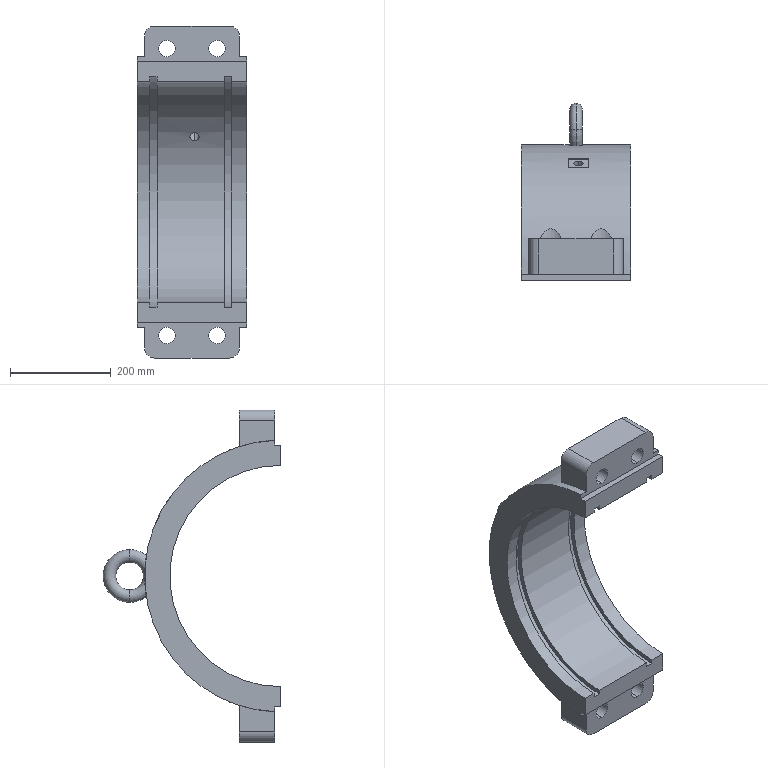Part | SolidWorks | features ICE 5, 3DProfileFeature 1, Extrusion 1, Fillet 1, HoleWzd 1, MirrorPattern 1, RevCut 1, Revolution 1 | 1 solid | 55 faces | box 218 x 352.5 x 660 mm | volume 9674169 mm3 | cylinder 26 | plane 25 | torus 4 | commonest cylinder face diameters 33 x8 70 x6 40 x4 440 x3 18.5 x2 458 x2